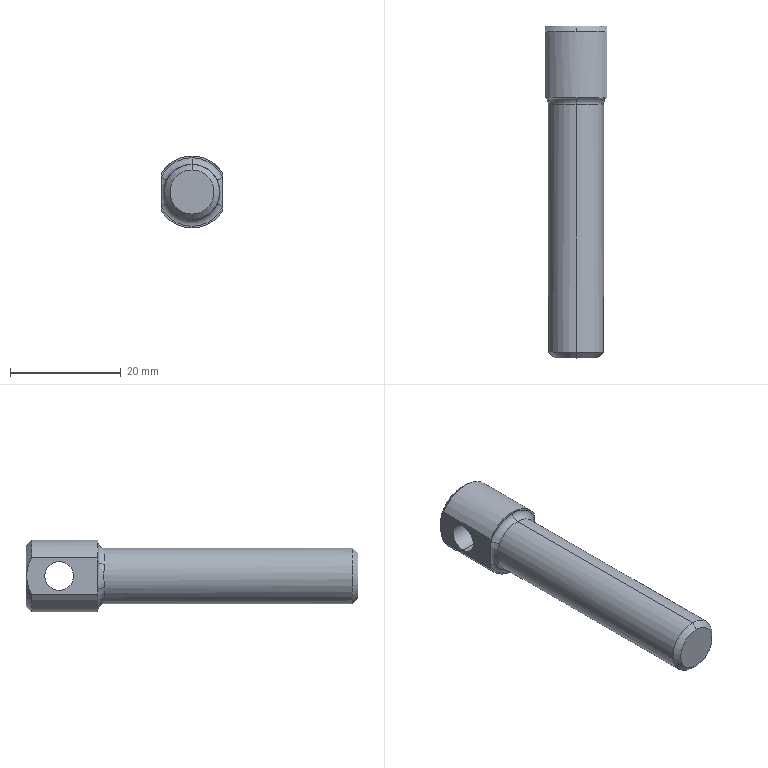Part | STEP file | 1 solid | 22 faces | box 11.2 x 60 x 13 mm | volume 5055 mm3 | cylinder 7 | plane 6 | cone 4 | torus 3 | spline 2 | commonest cylinder face diameters 13 x3 5.2 x2 10 x2